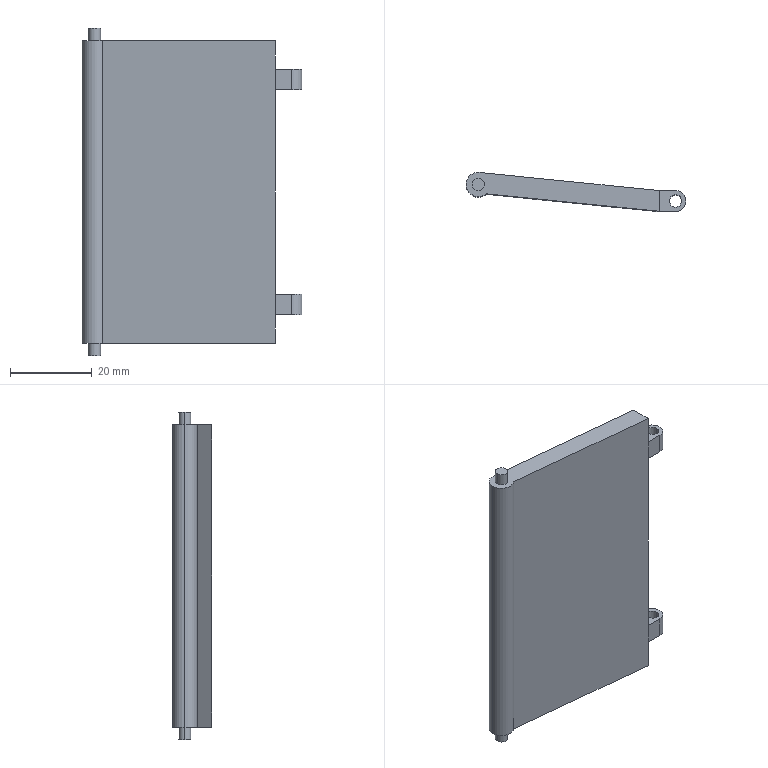Part | SolidWorks | features BaseBody 1 | 1 solid | 30 faces | box 53.735 x 9.545 x 80 mm | volume 17956 mm3 | plane 17 | cylinder 13 | commonest cylinder face diameters 3 x8 5.059 x3 6 x2
STEP:
#1=CARTESIAN_POINT('',(49.705,-4.016,25.));
#2=VERTEX_POINT('',#1);
#3=CARTESIAN_POINT('',(46.705,-4.016,25.));
#4=VERTEX_POINT('',#3);
#5=CARTESIAN_POINT('',(48.205,-4.016,25.));
#6=DIRECTION('',(0.,0.,-1.));
#7=DIRECTION('',(-1.,0.,0.));
#8=AXIS2_PLACEMENT_3D('',#5,#6,#7);
#9=CIRCLE('',#8,1.5);
#10=EDGE_CURVE('',#2,#4,#9,.T.);
#11=ORIENTED_EDGE('',*,*,#10,.T.);
#12=CARTESIAN_POINT('',(46.705,-4.016,30.));
#13=VERTEX_POINT('',#12);
#14=CARTESIAN_POINT('',(46.705,-4.016,-40.));
#15=DIRECTION('',(0.,0.,1.));
#16=VECTOR('',#15,1000.);
#17=LINE('',#14,#16);
#18=EDGE_CURVE('',#4,#13,#17,.T.);
#19=ORIENTED_EDGE('',*,*,#18,.T.);
#20=CARTESIAN_POINT('',(49.705,-4.016,30.));
#21=VERTEX_POINT('',#20);
#22=CARTESIAN_POINT('',(48.205,-4.016,30.));
#23=DIRECTION('',(0.,0.,1.));
#24=DIRECTION('',(1.,0.,0.));
#25=AXIS2_PLACEMENT_3D('',#22,#23,#24);
#26=CIRCLE('',#25,1.5);
#27=EDGE_CURVE('',#13,#21,#26,.T.);
#28=ORIENTED_EDGE('',*,*,#27,.T.);
#29=CARTESIAN_POINT('',(49.705,-4.016,-40.));
#30=DIRECTION('',(0.,0.,1.));
#31=VECTOR('',#30,1000.);
#32=LINE('',#29,#31);
#33=EDGE_CURVE('',#2,#21,#32,.T.);
#34=ORIENTED_EDGE('',*,*,#33,.F.);
#35=EDGE_LOOP('',(#11,#19,#28,#34));
#36=FACE_OUTER_BOUND('',#35,.T.);
#37=CARTESIAN_POINT('',(48.205,-4.016,-40.));
#38=DIRECTION('',(0.,0.,1.));
#39=DIRECTION('',(1.,0.,0.));
#40=AXIS2_PLACEMENT_3D('',#37,#38,#39);
#41=CYLINDRICAL_SURFACE('',#40,1.5);
#42=ADVANCED_FACE('',(#36),#41,.F.);
#43=CARTESIAN_POINT('',(46.705,-4.016,-30.));
#44=VERTEX_POINT('',#43);
#45=CARTESIAN_POINT('',(49.705,-4.016,-30.));
#46=VERTEX_POINT('',#45);
#47=CARTESIAN_POINT('',(48.205,-4.016,-30.));
#48=DIRECTION('',(0.,0.,1.));
#49=DIRECTION('',(1.,0.,0.));
#50=AXIS2_PLACEMENT_3D('',#47,#48,#49);
#51=CIRCLE('',#50,1.5);
#52=EDGE_CURVE('',#44,#46,#51,.T.);
#53=ORIENTED_EDGE('',*,*,#52,.F.);
#54=CARTESIAN_POINT('',(46.705,-4.016,-25.));
#55=VERTEX_POINT('',#54);
#56=CARTESIAN_POINT('',(46.705,-4.016,-40.));
#57=DIRECTION('',(0.,0.,1.));
#58=VECTOR('',#57,1000.);
#59=LINE('',#56,#58);
#60=EDGE_CURVE('',#44,#55,#59,.T.);
#61=ORIENTED_EDGE('',*,*,#60,.T.);
#62=CARTESIAN_POINT('',(49.705,-4.016,-25.));
#63=VERTEX_POINT('',#62);
#64=CARTESIAN_POINT('',(48.205,-4.016,-25.));
#65=DIRECTION('',(0.,0.,1.));
#66=DIRECTION('',(1.,0.,0.));
#67=AXIS2_PLACEMENT_3D('',#64,#65,#66);
#68=CIRCLE('',#67,1.5);
#69=EDGE_CURVE('',#55,#63,#68,.T.);
#70=ORIENTED_EDGE('',*,*,#69,.T.);
#71=CARTESIAN_POINT('',(49.705,-4.016,-40.));
#72=DIRECTION('',(0.,0.,1.));
#73=VECTOR('',#72,1000.);
#74=LINE('',#71,#73);
#75=EDGE_CURVE('',#46,#63,#74,.T.);
#76=ORIENTED_EDGE('',*,*,#75,.F.);
#77=EDGE_LOOP('',(#53,#61,#70,#76));
#78=FACE_OUTER_BOUND('',#77,.T.);
#79=CARTESIAN_POINT('',(48.205,-4.016,-40.));
#80=DIRECTION('',(0.,0.,1.));
#81=DIRECTION('',(1.,0.,0.));
#82=AXIS2_PLACEMENT_3D('',#79,#80,#81);
#83=CYLINDRICAL_SURFACE('',#82,1.5);
#84=ADVANCED_FACE('',(#78),#83,.F.);
#85=CARTESIAN_POINT('',(48.205,-6.545,-30.));
#86=VERTEX_POINT('',#85);
#87=CARTESIAN_POINT('',(50.735,-4.016,-30.));
#88=VERTEX_POINT('',#87);
#89=CARTESIAN_POINT('',(48.205,-4.016,-30.));
#90=DIRECTION('',(0.,0.,1.));
#91=DIRECTION('',(-1.,0.,0.));
#92=AXIS2_PLACEMENT_3D('',#89,#90,#91);
#93=CIRCLE('',#92,2.53);
#94=EDGE_CURVE('',#86,#88,#93,.T.);
#95=ORIENTED_EDGE('',*,*,#94,.T.);
#96=CARTESIAN_POINT('',(50.735,-4.016,-25.));
#97=VERTEX_POINT('',#96);
#98=CARTESIAN_POINT('',(50.735,-4.016,-30.));
#99=DIRECTION('',(0.,0.,1.));
#100=VECTOR('',#99,1000.);
#101=LINE('',#98,#100);
#102=EDGE_CURVE('',#88,#97,#101,.T.);
#103=ORIENTED_EDGE('',*,*,#102,.T.);
#104=CARTESIAN_POINT('',(48.205,-6.545,-25.));
#105=VERTEX_POINT('',#104);
#106=CARTESIAN_POINT('',(48.205,-4.016,-25.));
#107=DIRECTION('',(0.,0.,1.));
#108=DIRECTION('',(-1.,0.,0.));
#109=AXIS2_PLACEMENT_3D('',#106,#107,#108);
#110=CIRCLE('',#109,2.53);
#111=EDGE_CURVE('',#105,#97,#110,.T.);
#112=ORIENTED_EDGE('',*,*,#111,.F.);
#113=CARTESIAN_POINT('',(48.205,-6.545,-30.));
#114=DIRECTION('',(0.,0.,1.));
#115=VECTOR('',#114,1000.);
#116=LINE('',#113,#115);
#117=EDGE_CURVE('',#86,#105,#116,.T.);
#118=ORIENTED_EDGE('',*,*,#117,.F.);
#119=EDGE_LOOP('',(#95,#103,#112,#118));
#120=FACE_OUTER_BOUND('',#119,.T.);
#121=CARTESIAN_POINT('',(48.205,-4.016,-30.));
#122=DIRECTION('',(0.,0.,1.));
#123=DIRECTION('',(1.,0.,0.));
#124=AXIS2_PLACEMENT_3D('',#121,#122,#123);
#125=CYLINDRICAL_SURFACE('',#124,2.53);
#126=ADVANCED_FACE('',(#120),#125,.T.);
#127=CARTESIAN_POINT('',(1.5,0.,40.));
#128=VERTEX_POINT('',#127);
#129=CARTESIAN_POINT('',(-1.5,0.,40.));
#130=VERTEX_POINT('',#129);
#131=CARTESIAN_POINT('',(0.,0.,40.));
#132=DIRECTION('',(0.,0.,1.));
#133=DIRECTION('',(1.,0.,0.));
#134=AXIS2_PLACEMENT_3D('',#131,#132,#133);
#135=CIRCLE('',#134,1.5);
#136=EDGE_CURVE('',#128,#130,#135,.T.);
#137=ORIENTED_EDGE('',*,*,#136,.F.);
#138=CARTESIAN_POINT('',(1.5,0.,37.));
#139=VERTEX_POINT('',#138);
#140=CARTESIAN_POINT('',(1.5,0.,40.));
#141=DIRECTION('',(0.,0.,-1.));
#142=VECTOR('',#141,1000.);
#143=LINE('',#140,#142);
#144=EDGE_CURVE('',#128,#139,#143,.T.);
#145=ORIENTED_EDGE('',*,*,#144,.T.);
#146=CARTESIAN_POINT('',(-1.5,0.,37.));
#147=VERTEX_POINT('',#146);
#148=CARTESIAN_POINT('',(0.,0.,37.));
#149=DIRECTION('',(0.,0.,-1.));
#150=DIRECTION('',(1.,0.,0.));
#151=AXIS2_PLACEMENT_3D('',#148,#149,#150);
#152=CIRCLE('',#151,1.5);
#153=EDGE_CURVE('',#147,#139,#152,.T.);
#154=ORIENTED_EDGE('',*,*,#153,.F.);
#155=CARTESIAN_POINT('',(-1.5,0.,40.));
#156=DIRECTION('',(0.,0.,-1.));
#157=VECTOR('',#156,1000.);
#158=LINE('',#155,#157);
#159=EDGE_CURVE('',#130,#147,#158,.T.);
#160=ORIENTED_EDGE('',*,*,#159,.F.);
#161=EDGE_LOOP('',(#137,#145,#154,#160));
#162=FACE_OUTER_BOUND('',#161,.T.);
#163=CARTESIAN_POINT('',(0.,0.,40.));
#164=DIRECTION('',(0.,0.,-1.));
#165=DIRECTION('',(-1.,0.,0.));
#166=AXIS2_PLACEMENT_3D('',#163,#164,#165);
#167=CYLINDRICAL_SURFACE('',#166,1.5);
#168=ADVANCED_FACE('',(#162),#167,.T.);
#169=CARTESIAN_POINT('',(-1.5,0.,-37.));
#170=VERTEX_POINT('',#169);
#171=CARTESIAN_POINT('',(1.5,0.,-37.));
#172=VERTEX_POINT('',#171);
#173=CARTESIAN_POINT('',(0.,0.,-37.));
#174=DIRECTION('',(0.,0.,-1.));
#175=DIRECTION('',(1.,0.,0.));
#176=AXIS2_PLACEMENT_3D('',#173,#174,#175);
#177=CIRCLE('',#176,1.5);
#178=EDGE_CURVE('',#170,#172,#177,.T.);
#179=ORIENTED_EDGE('',*,*,#178,.T.);
#180=CARTESIAN_POINT('',(1.5,0.,-40.));
#181=VERTEX_POINT('',#180);
#182=CARTESIAN_POINT('',(1.5,0.,40.));
#183=DIRECTION('',(0.,0.,-1.));
#184=VECTOR('',#183,1000.);
#185=LINE('',#182,#184);
#186=EDGE_CURVE('',#172,#181,#185,.T.);
#187=ORIENTED_EDGE('',*,*,#186,.T.);
#188=CARTESIAN_POINT('',(-1.5,0.,-40.));
#189=VERTEX_POINT('',#188);
#190=CARTESIAN_POINT('',(0.,0.,-40.));
#191=DIRECTION('',(0.,0.,1.));
#192=DIRECTION('',(1.,0.,0.));
#193=AXIS2_PLACEMENT_3D('',#190,#191,#192);
#194=CIRCLE('',#193,1.5);
#195=EDGE_CURVE('',#181,#189,#194,.T.);
#196=ORIENTED_EDGE('',*,*,#195,.T.);
#197=CARTESIAN_POINT('',(-1.5,0.,40.));
#198=DIRECTION('',(0.,0.,-1.));
#199=VECTOR('',#198,1000.);
#200=LINE('',#197,#199);
#201=EDGE_CURVE('',#170,#189,#200,.T.);
#202=ORIENTED_EDGE('',*,*,#201,.F.);
#203=EDGE_LOOP('',(#179,#187,#196,#202));
#204=FACE_OUTER_BOUND('',#203,.T.);
#205=CARTESIAN_POINT('',(0.,0.,40.));
#206=DIRECTION('',(0.,0.,-1.));
#207=DIRECTION('',(-1.,0.,0.));
#208=AXIS2_PLACEMENT_3D('',#205,#206,#207);
#209=CYLINDRICAL_SURFACE('',#208,1.5);
#210=ADVANCED_FACE('',(#204),#209,.T.);
#211=CARTESIAN_POINT('',(-3.,0.,37.));
#212=VERTEX_POINT('',#211);
#213=CARTESIAN_POINT('',(1.947,-2.282,37.));
#214=VERTEX_POINT('',#213);
#215=CARTESIAN_POINT('',(0.,0.,37.));
#216=DIRECTION('',(0.,0.,1.));
#217=DIRECTION('',(1.,0.,0.));
#218=AXIS2_PLACEMENT_3D('',#215,#216,#217);
#219=CIRCLE('',#218,3.);
#220=EDGE_CURVE('',#212,#214,#219,.T.);
#221=ORIENTED_EDGE('',*,*,#220,.F.);
#222=CARTESIAN_POINT('',(-3.,0.,-37.));
#223=VERTEX_POINT('',#222);
#224=CARTESIAN_POINT('',(-3.,0.,37.));
#225=DIRECTION('',(0.,0.,-1.));
#226=VECTOR('',#225,1000.);
#227=LINE('',#224,#226);
#228=EDGE_CURVE('',#212,#223,#227,.T.);
#229=ORIENTED_EDGE('',*,*,#228,.T.);
#230=CARTESIAN_POINT('',(1.947,-2.282,-37.));
#231=VERTEX_POINT('',#230);
#232=CARTESIAN_POINT('',(0.,0.,-37.));
#233=DIRECTION('',(0.,0.,1.));
#234=DIRECTION('',(1.,0.,0.));
#235=AXIS2_PLACEMENT_3D('',#232,#233,#234);
#236=CIRCLE('',#235,3.);
#237=EDGE_CURVE('',#223,#231,#236,.T.);
#238=ORIENTED_EDGE('',*,*,#237,.T.);
#239=CARTESIAN_POINT('',(1.947,-2.282,37.));
#240=DIRECTION('',(0.,0.,-1.));
#241=VECTOR('',#240,1000.);
#242=LINE('',#239,#241);
#243=EDGE_CURVE('',#214,#231,#242,.T.);
#244=ORIENTED_EDGE('',*,*,#243,.F.);
#245=EDGE_LOOP('',(#221,#229,#238,#244));
#246=FACE_OUTER_BOUND('',#245,.T.);
#247=CARTESIAN_POINT('',(0.,0.,37.));
#248=DIRECTION('',(0.,0.,-1.));
#249=DIRECTION('',(-1.,0.,0.));
#250=AXIS2_PLACEMENT_3D('',#247,#248,#249);
#251=CYLINDRICAL_SURFACE('',#250,3.);
#252=ADVANCED_FACE('',(#246),#251,.T.);
#253=CARTESIAN_POINT('',(44.205,-1.486,-30.));
#254=VERTEX_POINT('',#253);
#255=CARTESIAN_POINT('',(44.205,-6.545,-30.));
#256=VERTEX_POINT('',#255);
#257=CARTESIAN_POINT('',(44.205,-6.545,-30.));
#258=DIRECTION('',(0.,-1.,0.));
#259=VECTOR('',#258,1000.);
#260=LINE('',#257,#259);
#261=EDGE_CURVE('',#254,#256,#260,.T.);
#262=ORIENTED_EDGE('',*,*,#261,.T.);
#263=CARTESIAN_POINT('',(44.205,-6.545,-37.));
#264=VERTEX_POINT('',#263);
#265=CARTESIAN_POINT('',(44.205,-6.545,37.));
#266=DIRECTION('',(0.,0.,-1.));
#267=VECTOR('',#266,1000.);
#268=LINE('',#265,#267);
#269=EDGE_CURVE('',#256,#264,#268,.T.);
#270=ORIENTED_EDGE('',*,*,#269,.T.);
#271=CARTESIAN_POINT('',(44.205,-1.486,-37.));
#272=VERTEX_POINT('',#271);
#273=CARTESIAN_POINT('',(44.205,0.,-37.));
#274=DIRECTION('',(0.,1.,0.));
#275=VECTOR('',#274,1000.);
#276=LINE('',#273,#275);
#277=EDGE_CURVE('',#264,#272,#276,.T.);
#278=ORIENTED_EDGE('',*,*,#277,.T.);
#279=CARTESIAN_POINT('',(44.205,-1.486,37.));
#280=DIRECTION('',(0.,0.,-1.));
#281=VECTOR('',#280,1000.);
#282=LINE('',#279,#281);
#283=EDGE_CURVE('',#254,#272,#282,.T.);
#284=ORIENTED_EDGE('',*,*,#283,.F.);
#285=EDGE_LOOP('',(#262,#270,#278,#284));
#286=FACE_OUTER_BOUND('',#285,.T.);
#287=CARTESIAN_POINT('',(44.205,0.,37.));
#288=DIRECTION('',(-1.,0.,0.));
#289=DIRECTION('',(0.,0.,1.));
#290=AXIS2_PLACEMENT_3D('',#287,#288,#289);
#291=PLANE('',#290);
#292=ADVANCED_FACE('',(#286),#291,.F.);
#293=CARTESIAN_POINT('',(44.205,-1.486,30.));
#294=VERTEX_POINT('',#293);
#295=CARTESIAN_POINT('',(44.205,-6.545,30.));
#296=VERTEX_POINT('',#295);
#297=CARTESIAN_POINT('',(44.205,-6.545,30.));
#298=DIRECTION('',(0.,-1.,0.));
#299=VECTOR('',#298,1000.);
#300=LINE('',#297,#299);
#301=EDGE_CURVE('',#294,#296,#300,.T.);
#302=ORIENTED_EDGE('',*,*,#301,.F.);
#303=CARTESIAN_POINT('',(44.205,-1.486,37.));
#304=VERTEX_POINT('',#303);
#305=CARTESIAN_POINT('',(44.205,-1.486,37.));
#306=DIRECTION('',(0.,0.,-1.));
#307=VECTOR('',#306,1000.);
#308=LINE('',#305,#307);
#309=EDGE_CURVE('',#304,#294,#308,.T.);
#310=ORIENTED_EDGE('',*,*,#309,.F.);
#311=CARTESIAN_POINT('',(44.205,-6.545,37.));
#312=VERTEX_POINT('',#311);
#313=CARTESIAN_POINT('',(44.205,0.,37.));
#314=DIRECTION('',(0.,1.,0.));
#315=VECTOR('',#314,1000.);
#316=LINE('',#313,#315);
#317=EDGE_CURVE('',#312,#304,#316,.T.);
#318=ORIENTED_EDGE('',*,*,#317,.F.);
#319=CARTESIAN_POINT('',(44.205,-6.545,37.));
#320=DIRECTION('',(0.,0.,-1.));
#321=VECTOR('',#320,1000.);
#322=LINE('',#319,#321);
#323=EDGE_CURVE('',#312,#296,#322,.T.);
#324=ORIENTED_EDGE('',*,*,#323,.T.);
#325=EDGE_LOOP('',(#302,#310,#318,#324));
#326=FACE_OUTER_BOUND('',#325,.T.);
#327=CARTESIAN_POINT('',(44.205,0.,37.));
#328=DIRECTION('',(-1.,0.,0.));
#329=DIRECTION('',(0.,0.,1.));
#330=AXIS2_PLACEMENT_3D('',#327,#328,#329);
#331=PLANE('',#330);
#332=ADVANCED_FACE('',(#326),#331,.F.);
#333=ORIENTED_EDGE('',*,*,#228,.F.);
#334=CARTESIAN_POINT('',(0.7932,2.893,37.));
#335=VERTEX_POINT('',#334);
#336=CARTESIAN_POINT('',(0.,0.,37.));
#337=DIRECTION('',(0.,0.,1.));
#338=DIRECTION('',(1.,0.,0.));
#339=AXIS2_PLACEMENT_3D('',#336,#337,#338);
#340=CIRCLE('',#339,3.);
#341=EDGE_CURVE('',#335,#212,#340,.T.);
#342=ORIENTED_EDGE('',*,*,#341,.F.);
#343=CARTESIAN_POINT('',(0.7932,2.893,-37.));
#344=VERTEX_POINT('',#343);
#345=CARTESIAN_POINT('',(0.7932,2.893,37.));
#346=DIRECTION('',(0.,0.,-1.));
#347=VECTOR('',#346,1000.);
#348=LINE('',#345,#347);
#349=EDGE_CURVE('',#335,#344,#348,.T.);
#350=ORIENTED_EDGE('',*,*,#349,.T.);
#351=CARTESIAN_POINT('',(0.,0.,-37.));
#352=DIRECTION('',(0.,0.,1.));
#353=DIRECTION('',(1.,0.,0.));
#354=AXIS2_PLACEMENT_3D('',#351,#352,#353);
#355=CIRCLE('',#354,3.);
#356=EDGE_CURVE('',#344,#223,#355,.T.);
#357=ORIENTED_EDGE('',*,*,#356,.T.);
#358=EDGE_LOOP('',(#333,#342,#350,#357));
#359=FACE_OUTER_BOUND('',#358,.T.);
#360=CARTESIAN_POINT('',(0.,0.,37.));
#361=DIRECTION('',(0.,0.,-1.));
#362=DIRECTION('',(-1.,0.,0.));
#363=AXIS2_PLACEMENT_3D('',#360,#361,#362);
#364=CYLINDRICAL_SURFACE('',#363,3.);
#365=ADVANCED_FACE('',(#359),#364,.T.);
#366=ORIENTED_EDGE('',*,*,#153,.T.);
#367=CARTESIAN_POINT('',(0.,0.,37.));
#368=DIRECTION('',(0.,0.,-1.));
#369=DIRECTION('',(1.,0.,0.));
#370=AXIS2_PLACEMENT_3D('',#367,#368,#369);
#371=CIRCLE('',#370,1.5);
#372=EDGE_CURVE('',#139,#147,#371,.T.);
#373=ORIENTED_EDGE('',*,*,#372,.T.);
#374=EDGE_LOOP('',(#366,#373));
#375=FACE_BOUND('',#374,.T.);
#376=ORIENTED_EDGE('',*,*,#341,.T.);
#377=ORIENTED_EDGE('',*,*,#220,.T.);
#378=CARTESIAN_POINT('',(-0.2083,-2.065,37.));
#379=DIRECTION('',(0.995,-0.1004,0.));
#380=VECTOR('',#379,1000.);
#381=LINE('',#378,#380);
#382=EDGE_CURVE('',#214,#312,#381,.T.);
#383=ORIENTED_EDGE('',*,*,#382,.T.);
#384=ORIENTED_EDGE('',*,*,#317,.T.);
#385=CARTESIAN_POINT('',(0.2969,2.943,37.));
#386=DIRECTION('',(0.995,-0.1004,0.));
#387=VECTOR('',#386,1000.);
#388=LINE('',#385,#387);
#389=EDGE_CURVE('',#335,#304,#388,.T.);
#390=ORIENTED_EDGE('',*,*,#389,.F.);
#391=EDGE_LOOP('',(#376,#377,#383,#384,#390));
#392=FACE_OUTER_BOUND('',#391,.T.);
#393=CARTESIAN_POINT('',(0.,0.,37.));
#394=DIRECTION('',(0.,0.,1.));
#395=DIRECTION('',(1.,0.,0.));
#396=AXIS2_PLACEMENT_3D('',#393,#394,#395);
#397=PLANE('',#396);
#398=ADVANCED_FACE('',(#375,#392),#397,.T.);
#399=ORIENTED_EDGE('',*,*,#178,.F.);
#400=CARTESIAN_POINT('',(0.,0.,-37.));
#401=DIRECTION('',(0.,0.,-1.));
#402=DIRECTION('',(1.,0.,0.));
#403=AXIS2_PLACEMENT_3D('',#400,#401,#402);
#404=CIRCLE('',#403,1.5);
#405=EDGE_CURVE('',#172,#170,#404,.T.);
#406=ORIENTED_EDGE('',*,*,#405,.F.);
#407=EDGE_LOOP('',(#399,#406));
#408=FACE_BOUND('',#407,.T.);
#409=ORIENTED_EDGE('',*,*,#356,.F.);
#410=CARTESIAN_POINT('',(0.2969,2.943,-37.));
#411=DIRECTION('',(0.995,-0.1004,0.));
#412=VECTOR('',#411,1000.);
#413=LINE('',#410,#412);
#414=EDGE_CURVE('',#344,#272,#413,.T.);
#415=ORIENTED_EDGE('',*,*,#414,.T.);
#416=ORIENTED_EDGE('',*,*,#277,.F.);
#417=CARTESIAN_POINT('',(-0.2083,-2.065,-37.));
#418=DIRECTION('',(0.995,-0.1004,0.));
#419=VECTOR('',#418,1000.);
#420=LINE('',#417,#419);
#421=EDGE_CURVE('',#231,#264,#420,.T.);
#422=ORIENTED_EDGE('',*,*,#421,.F.);
#423=ORIENTED_EDGE('',*,*,#237,.F.);
#424=EDGE_LOOP('',(#409,#415,#416,#422,#423));
#425=FACE_OUTER_BOUND('',#424,.T.);
#426=CARTESIAN_POINT('',(0.,0.,-37.));
#427=DIRECTION('',(0.,0.,1.));
#428=DIRECTION('',(1.,0.,0.));
#429=AXIS2_PLACEMENT_3D('',#426,#427,#428);
#430=PLANE('',#429);
#431=ADVANCED_FACE('',(#408,#425),#430,.F.);
#432=ORIENTED_EDGE('',*,*,#421,.T.);
#433=ORIENTED_EDGE('',*,*,#269,.F.);
#434=CARTESIAN_POINT('',(44.205,-6.545,-25.));
#435=VERTEX_POINT('',#434);
#436=CARTESIAN_POINT('',(44.205,-6.545,-30.));
#437=DIRECTION('',(0.,0.,1.));
#438=VECTOR('',#437,1000.);
#439=LINE('',#436,#438);
#440=EDGE_CURVE('',#256,#435,#439,.T.);
#441=ORIENTED_EDGE('',*,*,#440,.T.);
#442=CARTESIAN_POINT('',(44.205,-6.545,25.));
#443=VERTEX_POINT('',#442);
#444=CARTESIAN_POINT('',(44.205,-6.545,37.));
#445=DIRECTION('',(0.,0.,-1.));
#446=VECTOR('',#445,1000.);
#447=LINE('',#444,#446);
#448=EDGE_CURVE('',#443,#435,#447,.T.);
#449=ORIENTED_EDGE('',*,*,#448,.F.);
#450=CARTESIAN_POINT('',(44.205,-6.545,30.));
#451=DIRECTION('',(0.,0.,-1.));
#452=VECTOR('',#451,1000.);
#453=LINE('',#450,#452);
#454=EDGE_CURVE('',#296,#443,#453,.T.);
#455=ORIENTED_EDGE('',*,*,#454,.F.);
#456=ORIENTED_EDGE('',*,*,#323,.F.);
#457=ORIENTED_EDGE('',*,*,#382,.F.);
#458=ORIENTED_EDGE('',*,*,#243,.T.);
#459=EDGE_LOOP('',(#432,#433,#441,#449,#455,#456,#457,#458));
#460=FACE_OUTER_BOUND('',#459,.T.);
#461=CARTESIAN_POINT('',(-0.2083,-2.065,37.));
#462=DIRECTION('',(0.1004,0.995,0.));
#463=DIRECTION('',(-0.995,0.1004,0.));
#464=AXIS2_PLACEMENT_3D('',#461,#462,#463);
#465=PLANE('',#464);
#466=ADVANCED_FACE('',(#460),#465,.F.);
#467=ORIENTED_EDGE('',*,*,#448,.T.);
#468=CARTESIAN_POINT('',(44.205,-1.486,-25.));
#469=VERTEX_POINT('',#468);
#470=CARTESIAN_POINT('',(44.205,-6.545,-25.));
#471=DIRECTION('',(0.,-1.,0.));
#472=VECTOR('',#471,1000.);
#473=LINE('',#470,#472);
#474=EDGE_CURVE('',#469,#435,#473,.T.);
#475=ORIENTED_EDGE('',*,*,#474,.F.);
#476=CARTESIAN_POINT('',(44.205,-1.486,25.));
#477=VERTEX_POINT('',#476);
#478=CARTESIAN_POINT('',(44.205,-1.486,37.));
#479=DIRECTION('',(0.,0.,-1.));
#480=VECTOR('',#479,1000.);
#481=LINE('',#478,#480);
#482=EDGE_CURVE('',#477,#469,#481,.T.);
#483=ORIENTED_EDGE('',*,*,#482,.F.);
#484=CARTESIAN_POINT('',(44.205,-6.545,25.));
#485=DIRECTION('',(0.,-1.,0.));
#486=VECTOR('',#485,1000.);
#487=LINE('',#484,#486);
#488=EDGE_CURVE('',#477,#443,#487,.T.);
#489=ORIENTED_EDGE('',*,*,#488,.T.);
#490=EDGE_LOOP('',(#467,#475,#483,#489));
#491=FACE_OUTER_BOUND('',#490,.T.);
#492=CARTESIAN_POINT('',(44.205,0.,37.));
#493=DIRECTION('',(-1.,0.,0.));
#494=DIRECTION('',(0.,0.,1.));
#495=AXIS2_PLACEMENT_3D('',#492,#493,#494);
#496=PLANE('',#495);
#497=ADVANCED_FACE('',(#491),#496,.F.);
#498=ORIENTED_EDGE('',*,*,#414,.F.);
#499=ORIENTED_EDGE('',*,*,#349,.F.);
#500=ORIENTED_EDGE('',*,*,#389,.T.);
#501=ORIENTED_EDGE('',*,*,#309,.T.);
#502=CARTESIAN_POINT('',(44.205,-1.486,30.));
#503=DIRECTION('',(0.,0.,-1.));
#504=VECTOR('',#503,1000.);
#505=LINE('',#502,#504);
#506=EDGE_CURVE('',#294,#477,#505,.T.);
#507=ORIENTED_EDGE('',*,*,#506,.T.);
#508=ORIENTED_EDGE('',*,*,#482,.T.);
#509=CARTESIAN_POINT('',(44.205,-1.486,-30.));
#510=DIRECTION('',(0.,0.,1.));
#511=VECTOR('',#510,1000.);
#512=LINE('',#509,#511);
#513=EDGE_CURVE('',#254,#469,#512,.T.);
#514=ORIENTED_EDGE('',*,*,#513,.F.);
#515=ORIENTED_EDGE('',*,*,#283,.T.);
#516=EDGE_LOOP('',(#498,#499,#500,#501,#507,#508,#514,#515));
#517=FACE_OUTER_BOUND('',#516,.T.);
#518=CARTESIAN_POINT('',(0.2969,2.943,37.));
#519=DIRECTION('',(0.1004,0.995,0.));
#520=DIRECTION('',(-0.995,0.1004,0.));
#521=AXIS2_PLACEMENT_3D('',#518,#519,#520);
#522=PLANE('',#521);
#523=ADVANCED_FACE('',(#517),#522,.T.);
#524=CARTESIAN_POINT('',(0.,0.,-40.));
#525=DIRECTION('',(0.,0.,1.));
#526=DIRECTION('',(1.,0.,0.));
#527=AXIS2_PLACEMENT_3D('',#524,#525,#526);
#528=CIRCLE('',#527,1.5);
#529=EDGE_CURVE('',#189,#181,#528,.T.);
#530=ORIENTED_EDGE('',*,*,#529,.F.);
#531=ORIENTED_EDGE('',*,*,#195,.F.);
#532=EDGE_LOOP('',(#530,#531));
#533=FACE_OUTER_BOUND('',#532,.T.);
#534=CARTESIAN_POINT('',(0.,0.,-40.));
#535=DIRECTION('',(0.,0.,1.));
#536=DIRECTION('',(1.,0.,0.));
#537=AXIS2_PLACEMENT_3D('',#534,#535,#536);
#538=PLANE('',#537);
#539=ADVANCED_FACE('',(#533),#538,.F.);
#540=ORIENTED_EDGE('',*,*,#186,.F.);
#541=ORIENTED_EDGE('',*,*,#405,.T.);
#542=ORIENTED_EDGE('',*,*,#201,.T.);
#543=ORIENTED_EDGE('',*,*,#529,.T.);
#544=EDGE_LOOP('',(#540,#541,#542,#543));
#545=FACE_OUTER_BOUND('',#544,.T.);
#546=CARTESIAN_POINT('',(0.,0.,40.));
#547=DIRECTION('',(0.,0.,-1.));
#548=DIRECTION('',(-1.,0.,0.));
#549=AXIS2_PLACEMENT_3D('',#546,#547,#548);
#550=CYLINDRICAL_SURFACE('',#549,1.5);
#551=ADVANCED_FACE('',(#545),#550,.T.);
#552=ORIENTED_EDGE('',*,*,#144,.F.);
#553=CARTESIAN_POINT('',(0.,0.,40.));
#554=DIRECTION('',(0.,0.,1.));
#555=DIRECTION('',(1.,0.,0.));
#556=AXIS2_PLACEMENT_3D('',#553,#554,#555);
#557=CIRCLE('',#556,1.5);
#558=EDGE_CURVE('',#130,#128,#557,.T.);
#559=ORIENTED_EDGE('',*,*,#558,.F.);
#560=ORIENTED_EDGE('',*,*,#159,.T.);
#561=ORIENTED_EDGE('',*,*,#372,.F.);
#562=EDGE_LOOP('',(#552,#559,#560,#561));
#563=FACE_OUTER_BOUND('',#562,.T.);
#564=CARTESIAN_POINT('',(0.,0.,40.));
#565=DIRECTION('',(0.,0.,-1.));
#566=DIRECTION('',(-1.,0.,0.));
#567=AXIS2_PLACEMENT_3D('',#564,#565,#566);
#568=CYLINDRICAL_SURFACE('',#567,1.5);
#569=ADVANCED_FACE('',(#563),#568,.T.);
#570=ORIENTED_EDGE('',*,*,#558,.T.);
#571=ORIENTED_EDGE('',*,*,#136,.T.);
#572=EDGE_LOOP('',(#570,#571));
#573=FACE_OUTER_BOUND('',#572,.T.);
#574=CARTESIAN_POINT('',(0.,0.,40.));
#575=DIRECTION('',(0.,0.,1.));
#576=DIRECTION('',(1.,0.,0.));
#577=AXIS2_PLACEMENT_3D('',#574,#575,#576);
#578=PLANE('',#577);
#579=ADVANCED_FACE('',(#573),#578,.T.);
#580=CARTESIAN_POINT('',(48.205,-6.545,25.));
#581=VERTEX_POINT('',#580);
#582=CARTESIAN_POINT('',(48.205,-6.545,25.));
#583=DIRECTION('',(1.,0.,0.));
#584=VECTOR('',#583,1000.);
#585=LINE('',#582,#584);
#586=EDGE_CURVE('',#443,#581,#585,.T.);
#587=ORIENTED_EDGE('',*,*,#586,.T.);
#588=CARTESIAN_POINT('',(48.205,-6.545,30.));
#589=VERTEX_POINT('',#588);
#590=CARTESIAN_POINT('',(48.205,-6.545,30.));
#591=DIRECTION('',(0.,0.,-1.));
#592=VECTOR('',#591,1000.);
#593=LINE('',#590,#592);
#594=EDGE_CURVE('',#589,#581,#593,.T.);
#595=ORIENTED_EDGE('',*,*,#594,.F.);
#596=CARTESIAN_POINT('',(48.205,-6.545,30.));
#597=DIRECTION('',(1.,0.,0.));
#598=VECTOR('',#597,1000.);
#599=LINE('',#596,#598);
#600=EDGE_CURVE('',#296,#589,#599,.T.);
#601=ORIENTED_EDGE('',*,*,#600,.F.);
#602=ORIENTED_EDGE('',*,*,#454,.T.);
#603=EDGE_LOOP('',(#587,#595,#601,#602));
#604=FACE_OUTER_BOUND('',#603,.T.);
#605=CARTESIAN_POINT('',(48.205,-6.545,30.));
#606=DIRECTION('',(0.,1.,0.));
#607=DIRECTION('',(0.,0.,1.));
#608=AXIS2_PLACEMENT_3D('',#605,#606,#607);
#609=PLANE('',#608);
#610=ADVANCED_FACE('',(#604),#609,.F.);
#611=CARTESIAN_POINT('',(48.205,-1.486,25.));
#612=VERTEX_POINT('',#611);
#613=CARTESIAN_POINT('',(48.205,-4.016,25.));
#614=DIRECTION('',(0.,0.,1.));
#615=DIRECTION('',(-1.,0.,0.));
#616=AXIS2_PLACEMENT_3D('',#613,#614,#615);
#617=CIRCLE('',#616,2.53);
#618=EDGE_CURVE('',#581,#612,#617,.T.);
#619=ORIENTED_EDGE('',*,*,#618,.T.);
#620=CARTESIAN_POINT('',(48.205,-1.486,30.));
#621=VERTEX_POINT('',#620);
#622=CARTESIAN_POINT('',(48.205,-1.486,30.));
#623=DIRECTION('',(0.,0.,-1.));
#624=VECTOR('',#623,1000.);
#625=LINE('',#622,#624);
#626=EDGE_CURVE('',#621,#612,#625,.T.);
#627=ORIENTED_EDGE('',*,*,#626,.F.);
#628=CARTESIAN_POINT('',(48.205,-4.016,30.));
#629=DIRECTION('',(0.,0.,1.));
#630=DIRECTION('',(-1.,0.,0.));
#631=AXIS2_PLACEMENT_3D('',#628,#629,#630);
#632=CIRCLE('',#631,2.53);
#633=EDGE_CURVE('',#589,#621,#632,.T.);
#634=ORIENTED_EDGE('',*,*,#633,.F.);
#635=ORIENTED_EDGE('',*,*,#594,.T.);
#636=EDGE_LOOP('',(#619,#627,#634,#635));
#637=FACE_OUTER_BOUND('',#636,.T.);
#638=CARTESIAN_POINT('',(48.205,-4.016,30.));
#639=DIRECTION('',(0.,0.,-1.));
#640=DIRECTION('',(-1.,0.,0.));
#641=AXIS2_PLACEMENT_3D('',#638,#639,#640);
#642=CYLINDRICAL_SURFACE('',#641,2.53);
#643=ADVANCED_FACE('',(#637),#642,.T.);
#644=CARTESIAN_POINT('',(44.205,-1.486,25.));
#645=DIRECTION('',(-1.,0.,0.));
#646=VECTOR('',#645,1000.);
#647=LINE('',#644,#646);
#648=EDGE_CURVE('',#612,#477,#647,.T.);
#649=ORIENTED_EDGE('',*,*,#648,.T.);
#650=ORIENTED_EDGE('',*,*,#506,.F.);
#651=CARTESIAN_POINT('',(44.205,-1.486,30.));
#652=DIRECTION('',(-1.,0.,0.));
#653=VECTOR('',#652,1000.);
#654=LINE('',#651,#653);
#655=EDGE_CURVE('',#621,#294,#654,.T.);
#656=ORIENTED_EDGE('',*,*,#655,.F.);
#657=ORIENTED_EDGE('',*,*,#626,.T.);
#658=EDGE_LOOP('',(#649,#650,#656,#657));
#659=FACE_OUTER_BOUND('',#658,.T.);
#660=CARTESIAN_POINT('',(44.205,-1.486,30.));
#661=DIRECTION('',(0.,-1.,0.));
#662=DIRECTION('',(0.,0.,-1.));
#663=AXIS2_PLACEMENT_3D('',#660,#661,#662);
#664=PLANE('',#663);
#665=ADVANCED_FACE('',(#659),#664,.F.);
#666=CARTESIAN_POINT('',(48.205,-4.016,30.));
#667=DIRECTION('',(0.,0.,1.));
#668=DIRECTION('',(1.,0.,0.));
#669=AXIS2_PLACEMENT_3D('',#666,#667,#668);
#670=CIRCLE('',#669,1.5);
#671=EDGE_CURVE('',#21,#13,#670,.T.);
#672=ORIENTED_EDGE('',*,*,#671,.F.);
#673=ORIENTED_EDGE('',*,*,#27,.F.);
#674=EDGE_LOOP('',(#672,#673));
#675=FACE_BOUND('',#674,.T.);
#676=ORIENTED_EDGE('',*,*,#301,.T.);
#677=ORIENTED_EDGE('',*,*,#600,.T.);
#678=ORIENTED_EDGE('',*,*,#633,.T.);
#679=ORIENTED_EDGE('',*,*,#655,.T.);
#680=EDGE_LOOP('',(#676,#677,#678,#679));
#681=FACE_OUTER_BOUND('',#680,.T.);
#682=CARTESIAN_POINT('',(48.205,-4.016,30.));
#683=DIRECTION('',(0.,0.,-1.));
#684=DIRECTION('',(-1.,0.,0.));
#685=AXIS2_PLACEMENT_3D('',#682,#683,#684);
#686=PLANE('',#685);
#687=ADVANCED_FACE('',(#675,#681),#686,.F.);
#688=ORIENTED_EDGE('',*,*,#10,.F.);
#689=CARTESIAN_POINT('',(48.205,-4.016,25.));
#690=DIRECTION('',(0.,0.,-1.));
#691=DIRECTION('',(-1.,0.,0.));
#692=AXIS2_PLACEMENT_3D('',#689,#690,#691);
#693=CIRCLE('',#692,1.5);
#694=EDGE_CURVE('',#4,#2,#693,.T.);
#695=ORIENTED_EDGE('',*,*,#694,.F.);
#696=EDGE_LOOP('',(#688,#695));
#697=FACE_BOUND('',#696,.T.);
#698=ORIENTED_EDGE('',*,*,#488,.F.);
#699=ORIENTED_EDGE('',*,*,#648,.F.);
#700=ORIENTED_EDGE('',*,*,#618,.F.);
#701=ORIENTED_EDGE('',*,*,#586,.F.);
#702=EDGE_LOOP('',(#698,#699,#700,#701));
#703=FACE_OUTER_BOUND('',#702,.T.);
#704=CARTESIAN_POINT('',(48.205,-4.016,25.));
#705=DIRECTION('',(0.,0.,-1.));
#706=DIRECTION('',(-1.,0.,0.));
#707=AXIS2_PLACEMENT_3D('',#704,#705,#706);
#708=PLANE('',#707);
#709=ADVANCED_FACE('',(#697,#703),#708,.T.);
#710=CARTESIAN_POINT('',(48.205,-1.486,-25.));
#711=VERTEX_POINT('',#710);
#712=CARTESIAN_POINT('',(44.205,-1.486,-25.));
#713=DIRECTION('',(-1.,0.,0.));
#714=VECTOR('',#713,1000.);
#715=LINE('',#712,#714);
#716=EDGE_CURVE('',#711,#469,#715,.T.);
#717=ORIENTED_EDGE('',*,*,#716,.F.);
#718=CARTESIAN_POINT('',(48.205,-1.486,-30.));
#719=VERTEX_POINT('',#718);
#720=CARTESIAN_POINT('',(48.205,-1.486,-30.));
#721=DIRECTION('',(0.,0.,1.));
#722=VECTOR('',#721,1000.);
#723=LINE('',#720,#722);
#724=EDGE_CURVE('',#719,#711,#723,.T.);
#725=ORIENTED_EDGE('',*,*,#724,.F.);
#726=CARTESIAN_POINT('',(44.205,-1.486,-30.));
#727=DIRECTION('',(-1.,0.,0.));
#728=VECTOR('',#727,1000.);
#729=LINE('',#726,#728);
#730=EDGE_CURVE('',#719,#254,#729,.T.);
#731=ORIENTED_EDGE('',*,*,#730,.T.);
#732=ORIENTED_EDGE('',*,*,#513,.T.);
#733=EDGE_LOOP('',(#717,#725,#731,#732));
#734=FACE_OUTER_BOUND('',#733,.T.);
#735=CARTESIAN_POINT('',(44.205,-1.486,-30.));
#736=DIRECTION('',(0.,1.,0.));
#737=DIRECTION('',(0.,0.,1.));
#738=AXIS2_PLACEMENT_3D('',#735,#736,#737);
#739=PLANE('',#738);
#740=ADVANCED_FACE('',(#734),#739,.T.);
#741=ORIENTED_EDGE('',*,*,#102,.F.);
#742=CARTESIAN_POINT('',(48.205,-4.016,-30.));
#743=DIRECTION('',(0.,0.,1.));
#744=DIRECTION('',(-1.,0.,0.));
#745=AXIS2_PLACEMENT_3D('',#742,#743,#744);
#746=CIRCLE('',#745,2.53);
#747=EDGE_CURVE('',#88,#719,#746,.T.);
#748=ORIENTED_EDGE('',*,*,#747,.T.);
#749=ORIENTED_EDGE('',*,*,#724,.T.);
#750=CARTESIAN_POINT('',(48.205,-4.016,-25.));
#751=DIRECTION('',(0.,0.,1.));
#752=DIRECTION('',(-1.,0.,0.));
#753=AXIS2_PLACEMENT_3D('',#750,#751,#752);
#754=CIRCLE('',#753,2.53);
#755=EDGE_CURVE('',#97,#711,#754,.T.);
#756=ORIENTED_EDGE('',*,*,#755,.F.);
#757=EDGE_LOOP('',(#741,#748,#749,#756));
#758=FACE_OUTER_BOUND('',#757,.T.);
#759=CARTESIAN_POINT('',(48.205,-4.016,-30.));
#760=DIRECTION('',(0.,0.,1.));
#761=DIRECTION('',(1.,0.,0.));
#762=AXIS2_PLACEMENT_3D('',#759,#760,#761);
#763=CYLINDRICAL_SURFACE('',#762,2.53);
#764=ADVANCED_FACE('',(#758),#763,.T.);
#765=CARTESIAN_POINT('',(48.205,-6.545,-25.));
#766=DIRECTION('',(1.,0.,0.));
#767=VECTOR('',#766,1000.);
#768=LINE('',#765,#767);
#769=EDGE_CURVE('',#435,#105,#768,.T.);
#770=ORIENTED_EDGE('',*,*,#769,.F.);
#771=ORIENTED_EDGE('',*,*,#440,.F.);
#772=CARTESIAN_POINT('',(48.205,-6.545,-30.));
#773=DIRECTION('',(1.,0.,0.));
#774=VECTOR('',#773,1000.);
#775=LINE('',#772,#774);
#776=EDGE_CURVE('',#256,#86,#775,.T.);
#777=ORIENTED_EDGE('',*,*,#776,.T.);
#778=ORIENTED_EDGE('',*,*,#117,.T.);
#779=EDGE_LOOP('',(#770,#771,#777,#778));
#780=FACE_OUTER_BOUND('',#779,.T.);
#781=CARTESIAN_POINT('',(48.205,-6.545,-30.));
#782=DIRECTION('',(0.,-1.,0.));
#783=DIRECTION('',(0.,0.,-1.));
#784=AXIS2_PLACEMENT_3D('',#781,#782,#783);
#785=PLANE('',#784);
#786=ADVANCED_FACE('',(#780),#785,.T.);
#787=CARTESIAN_POINT('',(48.205,-4.016,-30.));
#788=DIRECTION('',(0.,0.,1.));
#789=DIRECTION('',(1.,0.,0.));
#790=AXIS2_PLACEMENT_3D('',#787,#788,#789);
#791=CIRCLE('',#790,1.5);
#792=EDGE_CURVE('',#46,#44,#791,.T.);
#793=ORIENTED_EDGE('',*,*,#792,.T.);
#794=ORIENTED_EDGE('',*,*,#52,.T.);
#795=EDGE_LOOP('',(#793,#794));
#796=FACE_BOUND('',#795,.T.);
#797=ORIENTED_EDGE('',*,*,#261,.F.);
#798=ORIENTED_EDGE('',*,*,#730,.F.);
#799=ORIENTED_EDGE('',*,*,#747,.F.);
#800=ORIENTED_EDGE('',*,*,#94,.F.);
#801=ORIENTED_EDGE('',*,*,#776,.F.);
#802=EDGE_LOOP('',(#797,#798,#799,#800,#801));
#803=FACE_OUTER_BOUND('',#802,.T.);
#804=CARTESIAN_POINT('',(48.205,-4.016,-30.));
#805=DIRECTION('',(0.,0.,1.));
#806=DIRECTION('',(-1.,0.,0.));
#807=AXIS2_PLACEMENT_3D('',#804,#805,#806);
#808=PLANE('',#807);
#809=ADVANCED_FACE('',(#796,#803),#808,.F.);
#810=CARTESIAN_POINT('',(48.205,-4.016,-25.));
#811=DIRECTION('',(0.,0.,1.));
#812=DIRECTION('',(1.,0.,0.));
#813=AXIS2_PLACEMENT_3D('',#810,#811,#812);
#814=CIRCLE('',#813,1.5);
#815=EDGE_CURVE('',#63,#55,#814,.T.);
#816=ORIENTED_EDGE('',*,*,#815,.F.);
#817=ORIENTED_EDGE('',*,*,#69,.F.);
#818=EDGE_LOOP('',(#816,#817));
#819=FACE_BOUND('',#818,.T.);
#820=ORIENTED_EDGE('',*,*,#474,.T.);
#821=ORIENTED_EDGE('',*,*,#769,.T.);
#822=ORIENTED_EDGE('',*,*,#111,.T.);
#823=ORIENTED_EDGE('',*,*,#755,.T.);
#824=ORIENTED_EDGE('',*,*,#716,.T.);
#825=EDGE_LOOP('',(#820,#821,#822,#823,#824));
#826=FACE_OUTER_BOUND('',#825,.T.);
#827=CARTESIAN_POINT('',(48.205,-4.016,-25.));
#828=DIRECTION('',(0.,0.,1.));
#829=DIRECTION('',(-1.,0.,0.));
#830=AXIS2_PLACEMENT_3D('',#827,#828,#829);
#831=PLANE('',#830);
#832=ADVANCED_FACE('',(#819,#826),#831,.T.);
#833=ORIENTED_EDGE('',*,*,#60,.F.);
#834=ORIENTED_EDGE('',*,*,#792,.F.);
#835=ORIENTED_EDGE('',*,*,#75,.T.);
#836=ORIENTED_EDGE('',*,*,#815,.T.);
#837=EDGE_LOOP('',(#833,#834,#835,#836));
#838=FACE_OUTER_BOUND('',#837,.T.);
#839=CARTESIAN_POINT('',(48.205,-4.016,-40.));
#840=DIRECTION('',(0.,0.,1.));
#841=DIRECTION('',(1.,0.,0.));
#842=AXIS2_PLACEMENT_3D('',#839,#840,#841);
#843=CYLINDRICAL_SURFACE('',#842,1.5);
#844=ADVANCED_FACE('',(#838),#843,.F.);
#845=ORIENTED_EDGE('',*,*,#18,.F.);
#846=ORIENTED_EDGE('',*,*,#694,.T.);
#847=ORIENTED_EDGE('',*,*,#33,.T.);
#848=ORIENTED_EDGE('',*,*,#671,.T.);
#849=EDGE_LOOP('',(#845,#846,#847,#848));
#850=FACE_OUTER_BOUND('',#849,.T.);
#851=CARTESIAN_POINT('',(48.205,-4.016,-40.));
#852=DIRECTION('',(0.,0.,1.));
#853=DIRECTION('',(1.,0.,0.));
#854=AXIS2_PLACEMENT_3D('',#851,#852,#853);
#855=CYLINDRICAL_SURFACE('',#854,1.5);
#856=ADVANCED_FACE('',(#850),#855,.F.);
#857=CLOSED_SHELL('',(#42,#84,#126,#168,#210,#252,#292,#332,#365,#398,#431,#466,#497,#523,#539,#551,#569,#579,#610,#643,#665,#687,#709,#740,#764,#786,#809,#832,#844,#856));
#858=MANIFOLD_SOLID_BREP('',#857);
#859=CARTESIAN_POINT('',(0.,0.,0.));
#860=DIRECTION('',(0.,0.,1.));
#861=DIRECTION('',(1.,0.,0.));
#862=AXIS2_PLACEMENT_3D('',#859,#860,#861);
#863=(LENGTH_UNIT()NAMED_UNIT(*)SI_UNIT(.MILLI.,.METRE.));
#864=UNCERTAINTY_MEASURE_WITH_UNIT(LENGTH_MEASURE(0.00001),#863,'','');
#865=(NAMED_UNIT(*)PLANE_ANGLE_UNIT()SI_UNIT($,.RADIAN.));
#866=(NAMED_UNIT(*)SI_UNIT($,.STERADIAN.)SOLID_ANGLE_UNIT());
#867=(GEOMETRIC_REPRESENTATION_CONTEXT(3)GLOBAL_UNCERTAINTY_ASSIGNED_CONTEXT((#864))GLOBAL_UNIT_ASSIGNED_CONTEXT((#863,#865,#866))REPRESENTATION_CONTEXT('',''));
#868=ADVANCED_BREP_SHAPE_REPRESENTATION('',(#858,#862),#867);